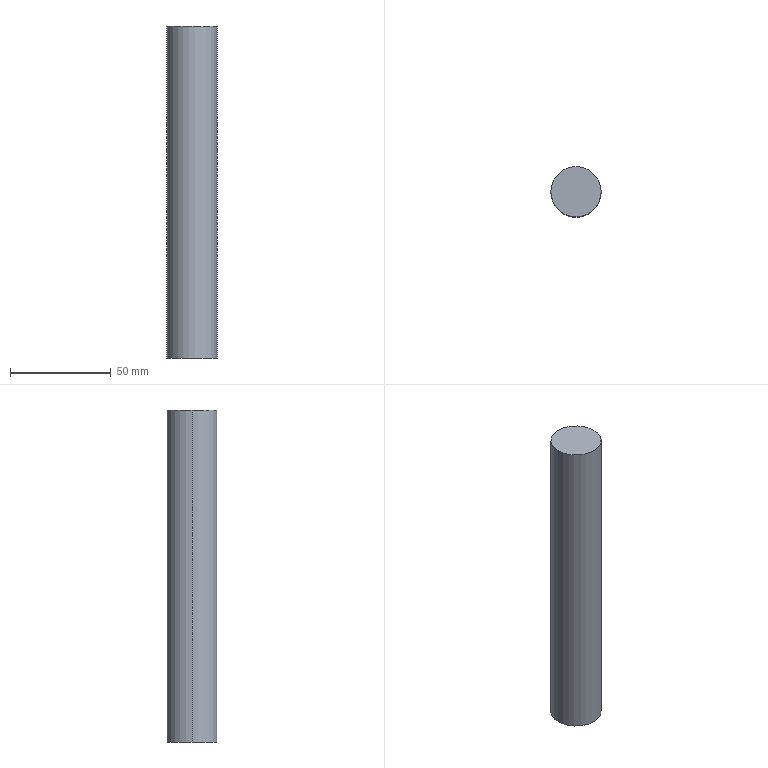Part | SolidWorks | features Extrusion 1 | 1 solid | 4 faces | box 25 x 25 x 165 mm | volume 80994 mm3 | cylinder 2 | plane 2 | commonest cylinder face diameters 25 x2
STEP:
#1=CARTESIAN_POINT('',(12.5,0.,165.));
#2=VERTEX_POINT('',#1);
#3=CARTESIAN_POINT('',(-12.5,0.,165.));
#4=VERTEX_POINT('',#3);
#5=CARTESIAN_POINT('',(0.,0.,165.));
#6=DIRECTION('',(0.,0.,1.));
#7=DIRECTION('',(1.,0.,0.));
#8=AXIS2_PLACEMENT_3D('',#5,#6,#7);
#9=CIRCLE('',#8,12.5);
#10=EDGE_CURVE('',#2,#4,#9,.T.);
#11=ORIENTED_EDGE('',*,*,#10,.F.);
#12=CARTESIAN_POINT('',(12.5,0.,0.));
#13=VERTEX_POINT('',#12);
#14=CARTESIAN_POINT('',(12.5,0.,165.));
#15=DIRECTION('',(0.,0.,-1.));
#16=VECTOR('',#15,1000.);
#17=LINE('',#14,#16);
#18=EDGE_CURVE('',#2,#13,#17,.T.);
#19=ORIENTED_EDGE('',*,*,#18,.T.);
#20=CARTESIAN_POINT('',(-12.5,0.,0.));
#21=VERTEX_POINT('',#20);
#22=CARTESIAN_POINT('',(0.,0.,0.));
#23=DIRECTION('',(0.,0.,1.));
#24=DIRECTION('',(1.,0.,0.));
#25=AXIS2_PLACEMENT_3D('',#22,#23,#24);
#26=CIRCLE('',#25,12.5);
#27=EDGE_CURVE('',#13,#21,#26,.T.);
#28=ORIENTED_EDGE('',*,*,#27,.T.);
#29=CARTESIAN_POINT('',(-12.5,0.,165.));
#30=DIRECTION('',(0.,0.,-1.));
#31=VECTOR('',#30,1000.);
#32=LINE('',#29,#31);
#33=EDGE_CURVE('',#4,#21,#32,.T.);
#34=ORIENTED_EDGE('',*,*,#33,.F.);
#35=EDGE_LOOP('',(#11,#19,#28,#34));
#36=FACE_OUTER_BOUND('',#35,.T.);
#37=CARTESIAN_POINT('',(0.,0.,165.));
#38=DIRECTION('',(0.,0.,-1.));
#39=DIRECTION('',(-1.,0.,0.));
#40=AXIS2_PLACEMENT_3D('',#37,#38,#39);
#41=CYLINDRICAL_SURFACE('',#40,12.5);
#42=ADVANCED_FACE('',(#36),#41,.T.);
#43=ORIENTED_EDGE('',*,*,#18,.F.);
#44=CARTESIAN_POINT('',(0.,0.,165.));
#45=DIRECTION('',(0.,0.,1.));
#46=DIRECTION('',(1.,0.,0.));
#47=AXIS2_PLACEMENT_3D('',#44,#45,#46);
#48=CIRCLE('',#47,12.5);
#49=EDGE_CURVE('',#4,#2,#48,.T.);
#50=ORIENTED_EDGE('',*,*,#49,.F.);
#51=ORIENTED_EDGE('',*,*,#33,.T.);
#52=CARTESIAN_POINT('',(0.,0.,0.));
#53=DIRECTION('',(0.,0.,1.));
#54=DIRECTION('',(1.,0.,0.));
#55=AXIS2_PLACEMENT_3D('',#52,#53,#54);
#56=CIRCLE('',#55,12.5);
#57=EDGE_CURVE('',#21,#13,#56,.T.);
#58=ORIENTED_EDGE('',*,*,#57,.T.);
#59=EDGE_LOOP('',(#43,#50,#51,#58));
#60=FACE_OUTER_BOUND('',#59,.T.);
#61=CARTESIAN_POINT('',(0.,0.,165.));
#62=DIRECTION('',(0.,0.,-1.));
#63=DIRECTION('',(-1.,0.,0.));
#64=AXIS2_PLACEMENT_3D('',#61,#62,#63);
#65=CYLINDRICAL_SURFACE('',#64,12.5);
#66=ADVANCED_FACE('',(#60),#65,.T.);
#67=ORIENTED_EDGE('',*,*,#49,.T.);
#68=ORIENTED_EDGE('',*,*,#10,.T.);
#69=EDGE_LOOP('',(#67,#68));
#70=FACE_OUTER_BOUND('',#69,.T.);
#71=CARTESIAN_POINT('',(0.,0.,165.));
#72=DIRECTION('',(0.,0.,1.));
#73=DIRECTION('',(1.,0.,0.));
#74=AXIS2_PLACEMENT_3D('',#71,#72,#73);
#75=PLANE('',#74);
#76=ADVANCED_FACE('',(#70),#75,.T.);
#77=ORIENTED_EDGE('',*,*,#57,.F.);
#78=ORIENTED_EDGE('',*,*,#27,.F.);
#79=EDGE_LOOP('',(#77,#78));
#80=FACE_OUTER_BOUND('',#79,.T.);
#81=CARTESIAN_POINT('',(0.,0.,0.));
#82=DIRECTION('',(0.,0.,1.));
#83=DIRECTION('',(1.,0.,0.));
#84=AXIS2_PLACEMENT_3D('',#81,#82,#83);
#85=PLANE('',#84);
#86=ADVANCED_FACE('',(#80),#85,.F.);
#87=CLOSED_SHELL('',(#42,#66,#76,#86));
#88=MANIFOLD_SOLID_BREP('',#87);
#89=CARTESIAN_POINT('',(0.,0.,0.));
#90=DIRECTION('',(0.,0.,1.));
#91=DIRECTION('',(1.,0.,0.));
#92=AXIS2_PLACEMENT_3D('',#89,#90,#91);
#93=(LENGTH_UNIT()NAMED_UNIT(*)SI_UNIT(.MILLI.,.METRE.));
#94=UNCERTAINTY_MEASURE_WITH_UNIT(LENGTH_MEASURE(0.00001),#93,'','');
#95=(NAMED_UNIT(*)PLANE_ANGLE_UNIT()SI_UNIT($,.RADIAN.));
#96=(NAMED_UNIT(*)SI_UNIT($,.STERADIAN.)SOLID_ANGLE_UNIT());
#97=(GEOMETRIC_REPRESENTATION_CONTEXT(3)GLOBAL_UNCERTAINTY_ASSIGNED_CONTEXT((#94))GLOBAL_UNIT_ASSIGNED_CONTEXT((#93,#95,#96))REPRESENTATION_CONTEXT('',''));
#98=ADVANCED_BREP_SHAPE_REPRESENTATION('',(#88,#92),#97);